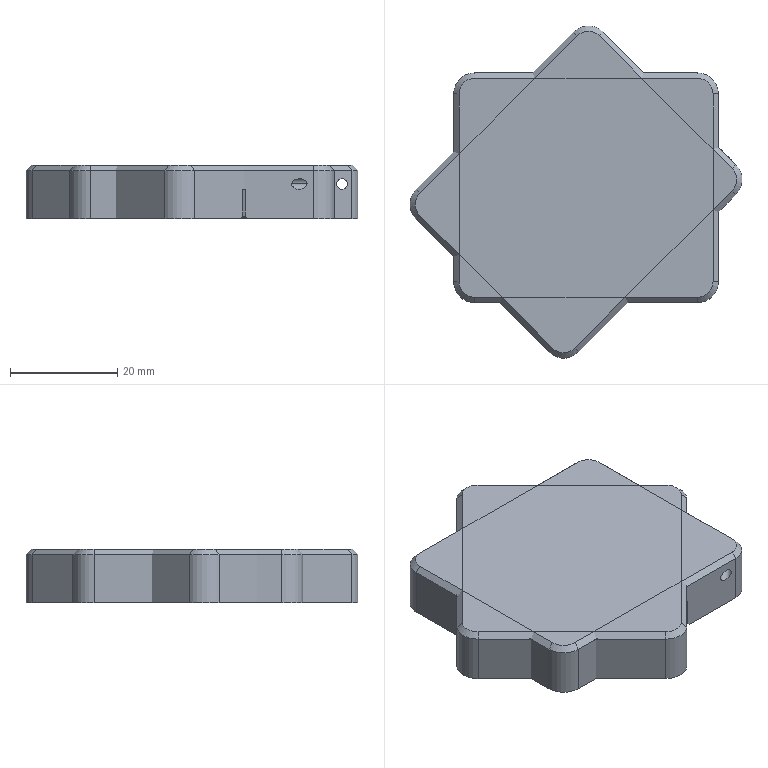Part | 2 solids | 98 faces | box 61.954 x 61.954 x 10 mm | volume 27577 mm3 | plane 46 | cylinder 36 | cone 16 | commonest cylinder face diameters 5 x16 7.86 x8 2 x4 10 x4 41 x4